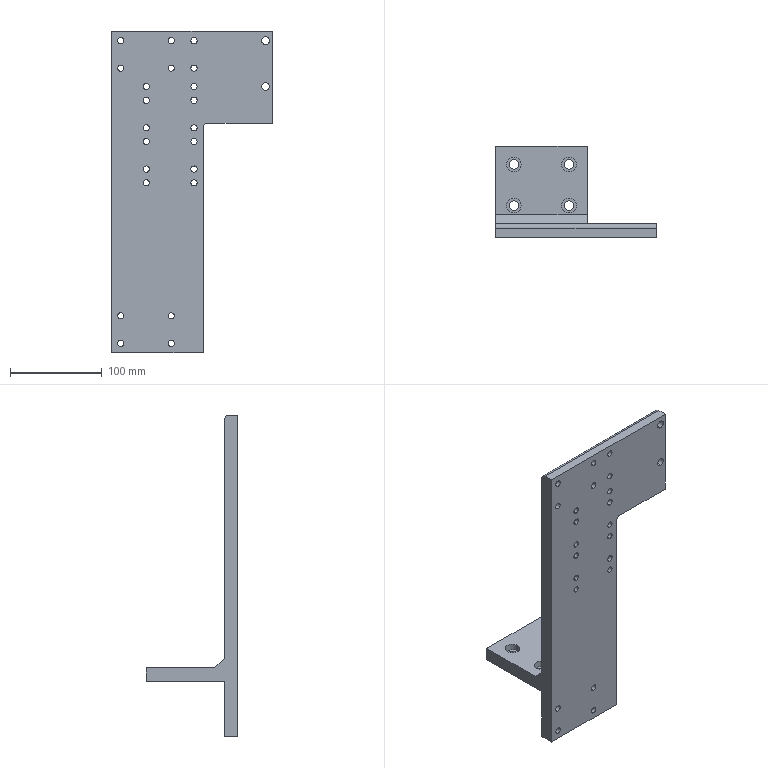Part | SolidWorks | features BaseBody 1 | 1 solid | 83 faces | box 175.5 x 100 x 350 mm | volume 747572 mm3 | cylinder 66 | plane 17 | commonest cylinder face diameters 6.8 x44 10.5 x8 16 x8 8.5 x4 10 x2